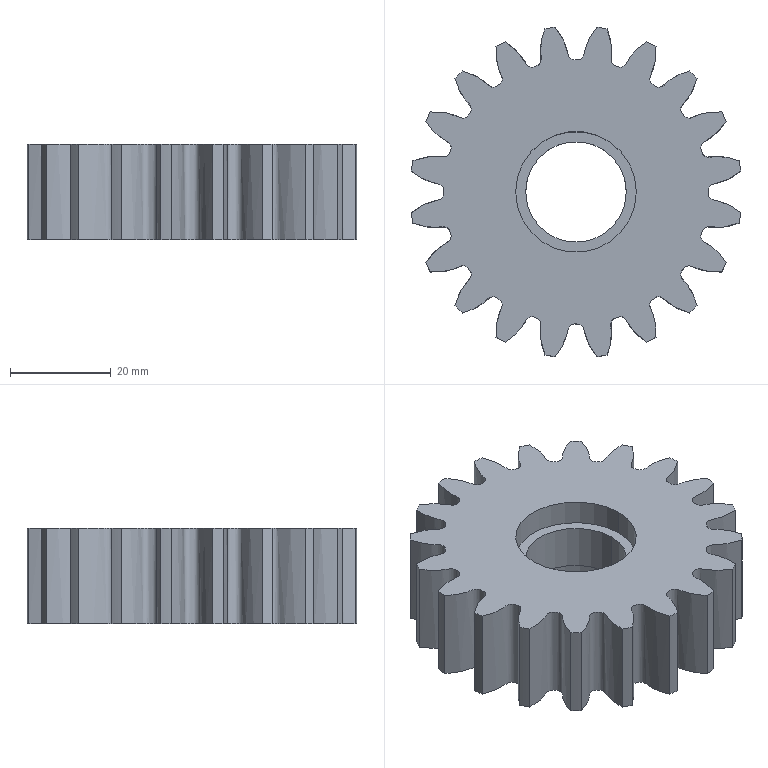Part | STEP file | Cuon T phu H01_18_Spur01 | 1 solid | 50 faces | box 65.481 x 65.481 x 19 mm | volume 46030 mm3 | cylinder 26 | spline 20 | plane 4 | commonest cylinder face diameters 66 x20 24 x4 20 x2